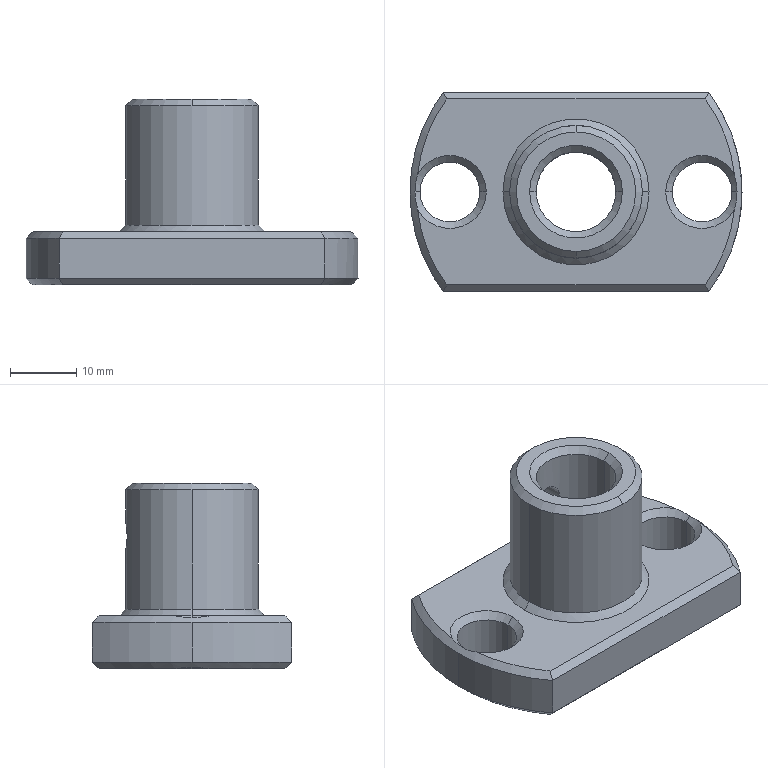Part | STEP file | SOP hanger seat | 1 solid | 43 faces | box 50 x 30 x 28 mm | volume 13038 mm3 | cone 21 | cylinder 13 | plane 9 | commonest cylinder face diameters 9 x4 50 x3 4.2 x2 12 x2 20 x2